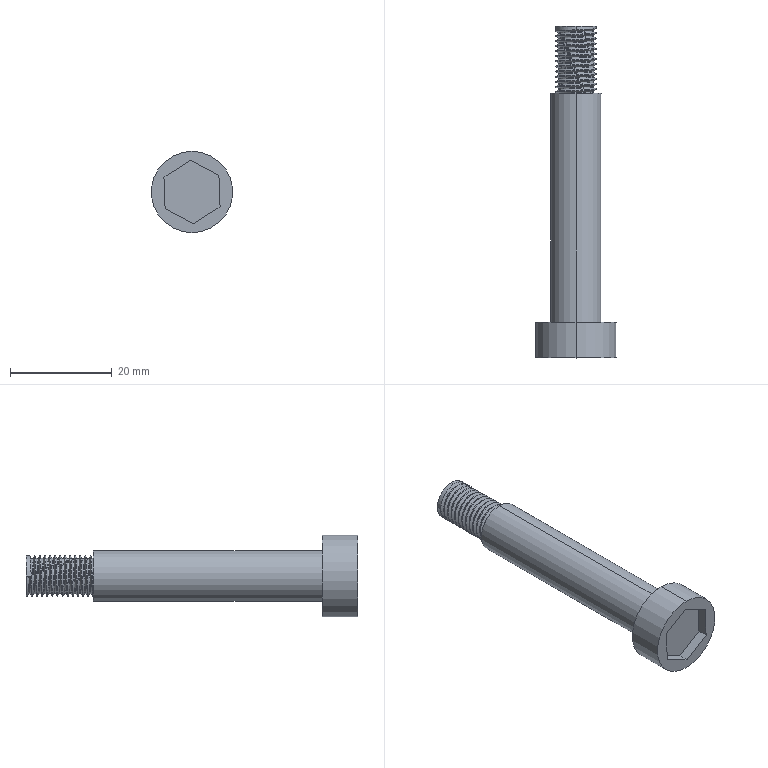Part | SolidWorks | features ICE 3, Extrusion 1, SweepThread 1 | 1 solid | 49 faces | box 16 x 65.25 x 16 mm | volume 5296 mm3 | cylinder 32 | plane 13 | spline 4 | commonest cylinder face diameters 8 x28 9.98 x2 16 x2